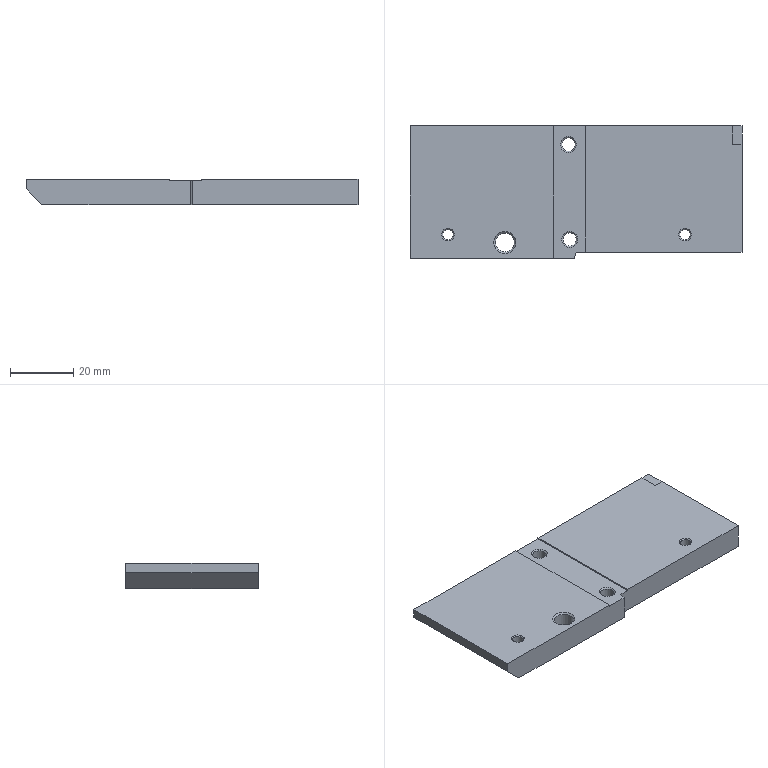NC program | NX | posted with a generic post | part box 105 x 42 x 8 mm
Whole program:
N10 G17 G21 G94 G90
(FLOOR_WALL_1_COPY_COPY , TOOL : D10)
N12 T10 M6
N14 G54
N16 G17 G0 G90 X-2.732 Y-10. B0. C0. S4500 M3
N18 G43 Z30. H10
N20 Z0.8
N22 G94 G1 Z-0.2 F1000.
N24 X-2.5 Y-9.866
N26 G3 X-2. Y-9. R1.
N28 G1 Y9. F1450.
N30 G3 X-2.5 Y9.866 R1.
N32 G1 X-2.732 Y10.
N34 Z0.8
N36 G0 Y-10. Z0.6
N38 G1 Z-0.4 F1000.
N40 X-2.5 Y-9.866
N42 G3 X-2. Y-9. R1.
N44 G1 Y9. F1450.
N46 G3 X-2.5 Y9.866 R1.
N48 G1 X-2.732 Y10.
N50 Z0.6
N52 G0 Y-10. Z0.4
N54 G1 Z-0.6 F1000.
N56 X-2.5 Y-9.866
N58 G3 X-2. Y-9. R1.
N60 G1 Y9. F1450.
N62 G3 X-2.5 Y9.866 R1.
N64 G1 X-2.732 Y10.
N66 Z0.4
N68 G0 Y-10. Z0.2
N70 G1 Z-0.8 F1000.
N72 X-2.5 Y-9.866
N74 G3 X-2. Y-9. R1.
N76 G1 Y9. F1450.
N78 G3 X-2.5 Y9.866 R1.
N80 G1 X-2.732 Y10.
N82 Z0.2
N84 G0 Y-10. Z0.
N86 G1 Z-1. F1000.
N88 X-2.5 Y-9.866
N90 G3 X-2. Y-9. R1.
N92 G1 Y9. F1450.
N94 G3 X-2.5 Y9.866 R1.
N96 G1 X-2.732 Y10.
N98 Z0.
N100 G0 Y-10. Z-0.2
N102 G1 Z-1.2 F1000.
N104 X-2.5 Y-9.866
N106 G3 X-2. Y-9. R1.
N108 G1 Y9. F1450.
N110 G3 X-2.5 Y9.866 R1.
N112 G1 X-2.732 Y10.
N114 Z-0.2
N116 G0 Y-10. Z-0.4
N118 G1 Z-1.4 F1000.
N120 X-2.5 Y-9.866
N122 G3 X-2. Y-9. R1.
N124 G1 Y9. F1450.
N126 G3 X-2.5 Y9.866 R1.
N128 G1 X-2.732 Y10.
N130 Z-0.4
N132 G0 Y-10. Z-0.6
N134 G1 Z-1.6 F1000.
N136 X-2.5 Y-9.866
N138 G3 X-2. Y-9. R1.
N140 G1 Y9. F1450.
N142 G3 X-2.5 Y9.866 R1.
N144 G1 X-2.732 Y10.
N146 Z-0.6
N148 G0 Y-10. Z-0.8
N150 G1 Z-1.8 F1000.
N152 X-2.5 Y-9.866
N154 G3 X-2. Y-9. R1.
N156 G1 Y9. F1450.
N158 G3 X-2.5 Y9.866 R1.
N160 G1 X-2.732 Y10.
N162 Z-0.8
N164 G0 Y-10. Z-1.
N166 G1 Z-2. F1000.
N168 X-2.5 Y-9.866
N170 G3 X-2. Y-9. R1.
N172 G1 Y9. F1450.
N174 G3 X-2.5 Y9.866 R1.
N176 G1 X-2.732 Y10.
N178 Z-1.
N180 G0 Y-10. Z-1.2
N182 G1 Z-2.2 F1000.
N184 X-2.5 Y-9.866
N186 G3 X-2. Y-9. R1.
N188 G1 Y9. F1450.
N190 G3 X-2.5 Y9.866 R1.
N192 G1 X-2.732 Y10.
N194 Z-1.2
N196 G0 Y-10. Z-1.4
N198 G1 Z-2.4 F1000.
N200 X-2.5 Y-9.866
N202 G3 X-2. Y-9. R1.
N204 G1 Y9. F1450.
N206 G3 X-2.5 Y9.866 R1.
N208 G1 X-2.732 Y10.
N210 Z-1.4
N212 G0 Y-10. Z-1.6
N214 G1 Z-2.6 F1000.
N216 X-2.5 Y-9.866
N218 G3 X-2. Y-9. R1.
N220 G1 Y9. F1450.
N222 G3 X-2.5 Y9.866 R1.
N224 G1 X-2.732 Y10.
N226 Z-1.6
N228 G0 Y-10. Z-1.8
N230 G1 Z-2.8 F1000.
N232 X-2.5 Y-9.866
N234 G3 X-2. Y-9. R1.
N236 G1 Y9. F1450.
N238 G3 X-2.5 Y9.866 R1.
N240 G1 X-2.732 Y10.
N242 Z-1.8
N244 G0 Y-10. Z-2.
N246 G1 Z-3. F1000.
N248 X-2.5 Y-9.866
N250 G3 X-2. Y-9. R1.
N252 G1 Y9. F1450.
N254 G3 X-2.5 Y9.866 R1.
N256 G1 X-2.732 Y10.
N258 Z-2.
N260 G0 Y-10. Z-2.2
N262 G1 Z-3.2 F1000.
N264 X-2.5 Y-9.866
N266 G3 X-2. Y-9. R1.
N268 G1 Y9. F1450.
N270 G3 X-2.5 Y9.866 R1.
N272 G1 X-2.732 Y10.
N274 Z-2.2
N276 G0 Y-10. Z-2.4
N278 G1 Z-3.4 F1000.
N280 X-2.5 Y-9.866
N282 G3 X-2. Y-9. R1.
N284 G1 Y9. F1450.
N286 G3 X-2.5 Y9.866 R1.
N288 G1 X-2.732 Y10.
N290 Z-2.4
N292 G0 Y-10. Z-2.6
N294 G1 Z-3.6 F1000.
N296 X-2.5 Y-9.866
N298 G3 X-2. Y-9. R1.
N300 G1 Y9. F1450.
N302 G3 X-2.5 Y9.866 R1.
N304 G1 X-2.732 Y10.
N306 Z-2.6
N308 G0 Y-10. Z-2.8
N310 G1 Z-3.8 F1000.
N312 X-2.5 Y-9.866
N314 G3 X-2. Y-9. R1.
N316 G1 Y9. F1450.
N318 G3 X-2.5 Y9.866 R1.
N320 G1 X-2.732 Y10.
N322 Z-2.8
N324 G0 Y-10. Z-3.
N326 G1 Z-4. F1000.
N328 X-2.5 Y-9.866
N330 G3 X-2. Y-9. R1.
N332 G1 Y9. F1450.
N334 G3 X-2.5 Y9.866 R1.
N336 G1 X-2.732 Y10.
N338 Z-3.
N340 G0 Y-10. Z-3.2
N342 G1 Z-4.2 F1000.
N344 X-2.5 Y-9.866
N346 G3 X-2. Y-9. R1.
N348 G1 Y9. F1450.
N350 G3 X-2.5 Y9.866 R1.
N352 G1 X-2.732 Y10.
N354 Z-3.2
N356 G0 Y-10. Z-3.4
N358 G1 Z-4.4 F1000.
N360 X-2.5 Y-9.866
N362 G3 X-2. Y-9. R1.
N364 G1 Y9. F1450.
N366 G3 X-2.5 Y9.866 R1.
N368 G1 X-2.732 Y10.
N370 Z-3.4
N372 G0 Y-10. Z-3.6
N374 G1 Z-4.6 F1000.
N376 X-2.5 Y-9.866
N378 G3 X-2. Y-9. R1.
N380 G1 Y9. F1450.
N382 G3 X-2.5 Y9.866 R1.
N384 G1 X-2.732 Y10.
N386 Z-3.6
N388 G0 Y-10. Z-3.8
N390 G1 Z-4.8 F1000.
N392 X-2.5 Y-9.866
N394 G3 X-2. Y-9. R1.
N396 G1 Y9. F1450.
N398 G3 X-2.5 Y9.866 R1.
N400 G1 X-2.732 Y10.
N402 Z-3.8
N404 G0 Y-10. Z-4.
N406 G1 Z-5. F1000.
N408 X-2.5 Y-9.866
N410 G3 X-2. Y-9. R1.
N412 G1 Y9. F1450.
N414 G3 X-2.5 Y9.866 R1.
N416 G1 X-2.732 Y10.
N418 Z-4.
N420 G0 Y-10. Z-4.2
N422 G1 Z-5.2 F1000.
N424 X-2.5 Y-9.866
N426 G3 X-2. Y-9. R1.
N428 G1 Y9. F1450.
N430 G3 X-2.5 Y9.866 R1.
N432 G1 X-2.732 Y10.
N434 Z-4.2
N436 G0 Y-10. Z-4.4
N438 G1 Z-5.4 F1000.
N440 X-2.5 Y-9.866
N442 G3 X-2. Y-9. R1.
N444 G1 Y9. F1450.
N446 G3 X-2.5 Y9.866 R1.
N448 G1 X-2.732 Y10.
N450 Z-4.4
N452 G0 Y-10. Z-4.6
N454 G1 Z-5.6 F1000.
N456 X-2.5 Y-9.866
N458 G3 X-2. Y-9. R1.
N460 G1 Y9. F1450.
N462 G3 X-2.5 Y9.866 R1.
N464 G1 X-2.732 Y10.
N466 Z-4.6
N468 G0 Y-10. Z-4.8
N470 G1 Z-5.8 F1000.
N472 X-2.5 Y-9.866
N474 G3 X-2. Y-9. R1.
N476 G1 Y9. F1450.
N478 G3 X-2.5 Y9.866 R1.
N480 G1 X-2.732 Y10.
N482 Z-4.8
N484 G0 Y-10. Z-5.
N486 G1 Z-6. F1000.
N488 X-2.5 Y-9.866
N490 G3 X-2. Y-9. R1.
N492 G1 Y9. F1450.
N494 G3 X-2.5 Y9.866 R1.
N496 G1 X-2.732 Y10.
N498 Z-5.
N500 G0 Z30.
N502 M5
(DRILLING_COPY_1 , TOOL : ZXZ)
N504 T02 M6
N506 G54
N508 G17 G0 G90 X75. Y0.3 B0. C0. S3000 M3
N510 G43 Z30. H2
N512 G94 G81 G98 Z-1. F250. R3.
N514 X16. Y-0.5
N516 X44.
N518 X89. Y0.3
N520 X97.
N522 G80
N524 G0 X97. Y0.3 Z30.
N526 M5
(DRILLING_COPY_COPY_1 , TOOL : 2.5ZT)
N528 T12 M6
N530 G54
N532 G17 G0 G90 X16. Y-0.5 B0. C0. S2000 M3
N534 G43 Z30. H12
N536 G94 G83 G98 Z-12.751 F120. Q2. R3.
N538 X44.
N540 X89. Y0.3
N542 X97.
N544 G80
N546 G0 X97. Y0.3 Z30.
N548 M5
(DRILLING_COPY_COPY_COPY_1 , TOOL : 4.2ZT)
N550 T14 M6
N552 G54
N554 G17 G0 G90 X75. Y0.3 B0. C0. S1929 M3
N556 G43 Z30. H14
N558 G94 G83 G98 Z-13.262 F120. Q2. R3.
N560 G80
N562 G0 X75. Y0.3 Z30.
N564 M5
(ZLEVEL_PROFILE_COPY_COPY_COPY_COPY_1 , TOOL : D6A45)
N566 T07 M6
N568 G54
N570 G17 G0 G90 X97. Y0.841 B0. C0. S6500 M3
N572 G43 Z30. H7
N574 Z1.
N576 G94 G1 Z-1. F1000.
N578 X96.998
N580 G3 X96.459 Y0.298 R0.541
N582 X97. Y0.841 R-0.541
N584 X96.74 Y0.691 R0.3
N586 G1 Z0.
N588 G0 Z30.
N590 X16. Y-1.041
N592 Z1.
N594 G1 Z-1.
N596 G3 X16.541 Y-0.5 R0.541
N598 X16. Y-1.041 R-0.541
N600 X16.26 Y-0.891 R0.3
N602 G1 Z0.
N604 G0 Z30.
N606 X44. Y-1.041
N608 Z1.
N610 G1 Z-1.
N612 G3 X44.541 Y-0.5 R0.541
N614 X44. Y-1.041 R-0.541
N616 X44.26 Y-0.891 R0.3
N618 G1 Z0.
N620 G0 Z30.
N622 X75.132 Y0.615
N624 Z0.
N626 G1 Z-1.
N628 X75.52 Y1.541
N630 G3 X75. Y1.841 R0.6
N632 X73.459 Y0.3 R1.541
N634 X75. Y1.841 R-1.541
N636 X74.48 Y1.541 R0.6
N638 G1 X74.868 Y0.615
N640 Z0.
N642 G0 Z30.
N644 X89. Y0.841
N646 Z1.
N648 G1 Z-1.
N650 G3 X88.459 Y0.3 R0.541
N652 X89. Y0.841 R-0.541
N654 X88.74 Y0.691 R0.3
N656 G1 Z0.
N658 G0 Z30.
N660 X100.921 Y-5.952
N662 Z0.
N664 G1 Z-1.
N666 X100.521 Y-5.259
N668 G3 X100.001 Y-4.959 R0.6
N670 G1 X2.999
N672 G2 X2.041 Y-4.001 R0.958
N674 G1 Y4.001
N676 G2 X2.999 Y4.959 R0.958
N678 G1 X49.501
N680 G2 X50.278 Y4.559 R0.967
N682 G1 X58.723
N684 G2 X59.499 Y4.959 R0.961
N686 G1 X105.001
N688 G2 X105.959 Y4.001 R0.967
N690 G1 Y0.999
N692 G2 X105.678 Y0.323 R0.957
N694 G1 X100.677 Y-4.678
N696 G2 X100.001 Y-4.959 R0.956
N698 G3 X99.481 Y-5.259 R0.6
N700 G1 X98.962 Y-6.159
N702 Z0.
N704 G0 Z30.
N706 M5
N708 M2